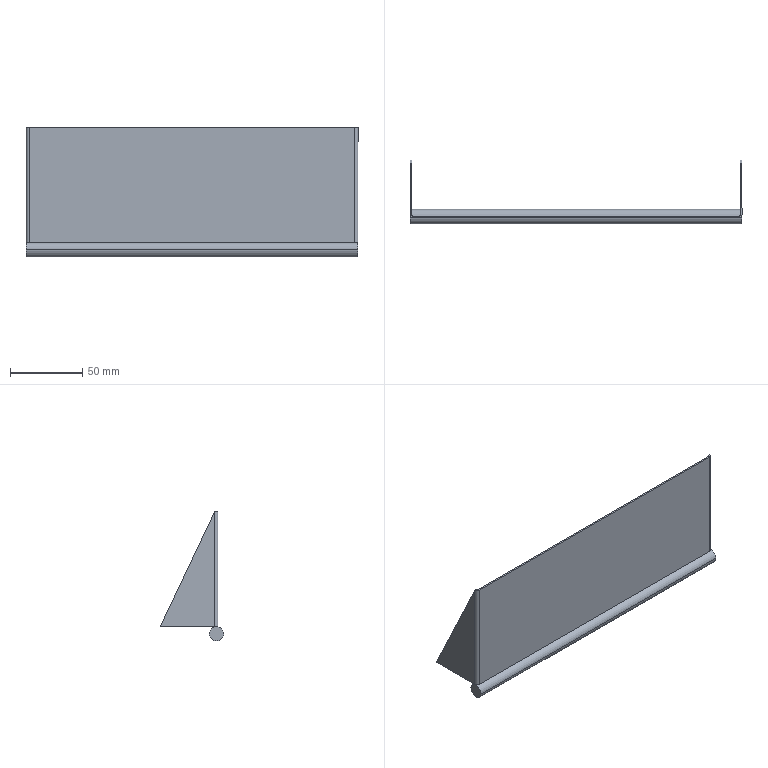Part | SolidWorks | features ICE 2, EdgeFlange 1, FlatPattern 1, SMBaseFlange 1, SheetMetal 1 | 2 solids | 24 faces | box 230 x 44 x 90 mm | volume 43833 mm3 | plane 18 | cylinder 6 | commonest cylinder face diameters 2 x2 4.4 x2 10 x2
STEP:
#1=CARTESIAN_POINT('',(112.8,-1.2,-40.));
#2=VERTEX_POINT('',#1);
#3=CARTESIAN_POINT('',(112.8,-1.2,40.));
#4=VERTEX_POINT('',#3);
#5=CARTESIAN_POINT('',(112.8,-1.2,-40.));
#6=DIRECTION('',(0.,0.,1.));
#7=VECTOR('',#6,1000.);
#8=LINE('',#5,#7);
#9=EDGE_CURVE('',#2,#4,#8,.T.);
#10=ORIENTED_EDGE('',*,*,#9,.T.);
#11=CARTESIAN_POINT('',(-112.8,-1.2,40.));
#12=VERTEX_POINT('',#11);
#13=CARTESIAN_POINT('',(-115.,-1.2,40.));
#14=DIRECTION('',(1.,0.,0.));
#15=VECTOR('',#14,1000.);
#16=LINE('',#13,#15);
#17=EDGE_CURVE('',#12,#4,#16,.T.);
#18=ORIENTED_EDGE('',*,*,#17,.F.);
#19=CARTESIAN_POINT('',(-112.8,-1.2,-40.));
#20=VERTEX_POINT('',#19);
#21=CARTESIAN_POINT('',(-112.8,-1.2,40.));
#22=DIRECTION('',(0.,0.,-1.));
#23=VECTOR('',#22,1000.);
#24=LINE('',#21,#23);
#25=EDGE_CURVE('',#12,#20,#24,.T.);
#26=ORIENTED_EDGE('',*,*,#25,.T.);
#27=CARTESIAN_POINT('',(-115.,-1.2,-40.));
#28=DIRECTION('',(-1.,0.,0.));
#29=VECTOR('',#28,1000.);
#30=LINE('',#27,#29);
#31=EDGE_CURVE('',#2,#20,#30,.T.);
#32=ORIENTED_EDGE('',*,*,#31,.F.);
#33=EDGE_LOOP('',(#10,#18,#26,#32));
#34=FACE_OUTER_BOUND('',#33,.T.);
#35=CARTESIAN_POINT('',(0.,-1.2,0.));
#36=DIRECTION('',(0.,1.,0.));
#37=DIRECTION('',(0.,0.,1.));
#38=AXIS2_PLACEMENT_3D('',#35,#36,#37);
#39=PLANE('',#38);
#40=ADVANCED_FACE('',(#34),#39,.F.);
#41=CARTESIAN_POINT('',(-112.8,0.,40.));
#42=VERTEX_POINT('',#41);
#43=CARTESIAN_POINT('',(112.8,0.,40.));
#44=VERTEX_POINT('',#43);
#45=CARTESIAN_POINT('',(-115.,0.,40.));
#46=DIRECTION('',(1.,0.,0.));
#47=VECTOR('',#46,1000.);
#48=LINE('',#45,#47);
#49=EDGE_CURVE('',#42,#44,#48,.T.);
#50=ORIENTED_EDGE('',*,*,#49,.T.);
#51=CARTESIAN_POINT('',(112.8,0.,-40.));
#52=VERTEX_POINT('',#51);
#53=CARTESIAN_POINT('',(112.8,0.,-40.));
#54=DIRECTION('',(0.,0.,1.));
#55=VECTOR('',#54,1000.);
#56=LINE('',#53,#55);
#57=EDGE_CURVE('',#52,#44,#56,.T.);
#58=ORIENTED_EDGE('',*,*,#57,.F.);
#59=CARTESIAN_POINT('',(-112.8,0.,-40.));
#60=VERTEX_POINT('',#59);
#61=CARTESIAN_POINT('',(-115.,0.,-40.));
#62=DIRECTION('',(-1.,0.,0.));
#63=VECTOR('',#62,1000.);
#64=LINE('',#61,#63);
#65=EDGE_CURVE('',#52,#60,#64,.T.);
#66=ORIENTED_EDGE('',*,*,#65,.T.);
#67=CARTESIAN_POINT('',(-112.8,0.,40.));
#68=DIRECTION('',(0.,0.,-1.));
#69=VECTOR('',#68,1000.);
#70=LINE('',#67,#69);
#71=EDGE_CURVE('',#42,#60,#70,.T.);
#72=ORIENTED_EDGE('',*,*,#71,.F.);
#73=EDGE_LOOP('',(#50,#58,#66,#72));
#74=FACE_OUTER_BOUND('',#73,.T.);
#75=CARTESIAN_POINT('',(0.,0.,0.));
#76=DIRECTION('',(0.,1.,0.));
#77=DIRECTION('',(0.,0.,1.));
#78=AXIS2_PLACEMENT_3D('',#75,#76,#77);
#79=PLANE('',#78);
#80=ADVANCED_FACE('',(#74),#79,.T.);
#81=ORIENTED_EDGE('',*,*,#65,.F.);
#82=CARTESIAN_POINT('',(112.8,0.,-40.));
#83=DIRECTION('',(0.,-1.,0.));
#84=VECTOR('',#83,1000.);
#85=LINE('',#82,#84);
#86=EDGE_CURVE('',#52,#2,#85,.T.);
#87=ORIENTED_EDGE('',*,*,#86,.T.);
#88=ORIENTED_EDGE('',*,*,#31,.T.);
#89=CARTESIAN_POINT('',(-112.8,0.,-40.));
#90=DIRECTION('',(0.,-1.,0.));
#91=VECTOR('',#90,1000.);
#92=LINE('',#89,#91);
#93=EDGE_CURVE('',#60,#20,#92,.T.);
#94=ORIENTED_EDGE('',*,*,#93,.F.);
#95=EDGE_LOOP('',(#81,#87,#88,#94));
#96=FACE_OUTER_BOUND('',#95,.T.);
#97=CARTESIAN_POINT('',(-115.,-1.2,-40.));
#98=DIRECTION('',(0.,0.,-1.));
#99=DIRECTION('',(-1.,0.,0.));
#100=AXIS2_PLACEMENT_3D('',#97,#98,#99);
#101=PLANE('',#100);
#102=ADVANCED_FACE('',(#96),#101,.T.);
#103=CARTESIAN_POINT('',(112.8,0.,40.));
#104=DIRECTION('',(0.,-1.,0.));
#105=VECTOR('',#104,1000.);
#106=LINE('',#103,#105);
#107=EDGE_CURVE('',#44,#4,#106,.T.);
#108=ORIENTED_EDGE('',*,*,#107,.F.);
#109=ORIENTED_EDGE('',*,*,#49,.F.);
#110=CARTESIAN_POINT('',(-112.8,0.,40.));
#111=DIRECTION('',(0.,-1.,0.));
#112=VECTOR('',#111,1000.);
#113=LINE('',#110,#112);
#114=EDGE_CURVE('',#42,#12,#113,.T.);
#115=ORIENTED_EDGE('',*,*,#114,.T.);
#116=ORIENTED_EDGE('',*,*,#17,.T.);
#117=EDGE_LOOP('',(#108,#109,#115,#116));
#118=FACE_OUTER_BOUND('',#117,.T.);
#119=CARTESIAN_POINT('',(-115.,-1.2,40.));
#120=DIRECTION('',(0.,0.,1.));
#121=DIRECTION('',(1.,0.,0.));
#122=AXIS2_PLACEMENT_3D('',#119,#120,#121);
#123=PLANE('',#122);
#124=ADVANCED_FACE('',(#118),#123,.T.);
#125=CARTESIAN_POINT('',(-113.8,1.,-40.));
#126=VERTEX_POINT('',#125);
#127=CARTESIAN_POINT('',(-115.,1.,-40.));
#128=VERTEX_POINT('',#127);
#129=CARTESIAN_POINT('',(-115.,1.,-40.));
#130=DIRECTION('',(-1.,0.,0.));
#131=VECTOR('',#130,1000.);
#132=LINE('',#129,#131);
#133=EDGE_CURVE('',#126,#128,#132,.T.);
#134=ORIENTED_EDGE('',*,*,#133,.F.);
#135=CARTESIAN_POINT('',(-112.8,1.,-40.));
#136=DIRECTION('',(0.,0.,-1.));
#137=DIRECTION('',(1.,0.,0.));
#138=AXIS2_PLACEMENT_3D('',#135,#136,#137);
#139=CIRCLE('',#138,1.);
#140=EDGE_CURVE('',#60,#126,#139,.T.);
#141=ORIENTED_EDGE('',*,*,#140,.F.);
#142=ORIENTED_EDGE('',*,*,#93,.T.);
#143=CARTESIAN_POINT('',(-112.8,1.,-40.));
#144=DIRECTION('',(0.,0.,-1.));
#145=DIRECTION('',(1.,0.,0.));
#146=AXIS2_PLACEMENT_3D('',#143,#144,#145);
#147=CIRCLE('',#146,2.2);
#148=EDGE_CURVE('',#20,#128,#147,.T.);
#149=ORIENTED_EDGE('',*,*,#148,.T.);
#150=EDGE_LOOP('',(#134,#141,#142,#149));
#151=FACE_OUTER_BOUND('',#150,.T.);
#152=CARTESIAN_POINT('',(-112.8,1.,-40.));
#153=DIRECTION('',(0.,0.,-1.));
#154=DIRECTION('',(-1.,0.,0.));
#155=AXIS2_PLACEMENT_3D('',#152,#153,#154);
#156=PLANE('',#155);
#157=ADVANCED_FACE('',(#151),#156,.T.);
#158=CARTESIAN_POINT('',(-113.8,1.,40.));
#159=VERTEX_POINT('',#158);
#160=CARTESIAN_POINT('',(-112.8,1.,40.));
#161=DIRECTION('',(0.,0.,1.));
#162=DIRECTION('',(1.,0.,0.));
#163=AXIS2_PLACEMENT_3D('',#160,#161,#162);
#164=CIRCLE('',#163,1.);
#165=EDGE_CURVE('',#159,#42,#164,.T.);
#166=ORIENTED_EDGE('',*,*,#165,.F.);
#167=CARTESIAN_POINT('',(-115.,1.,40.));
#168=VERTEX_POINT('',#167);
#169=CARTESIAN_POINT('',(-113.8,1.,40.));
#170=DIRECTION('',(-1.,0.,0.));
#171=VECTOR('',#170,1000.);
#172=LINE('',#169,#171);
#173=EDGE_CURVE('',#159,#168,#172,.T.);
#174=ORIENTED_EDGE('',*,*,#173,.T.);
#175=CARTESIAN_POINT('',(-112.8,1.,40.));
#176=DIRECTION('',(0.,0.,1.));
#177=DIRECTION('',(1.,0.,0.));
#178=AXIS2_PLACEMENT_3D('',#175,#176,#177);
#179=CIRCLE('',#178,2.2);
#180=EDGE_CURVE('',#168,#12,#179,.T.);
#181=ORIENTED_EDGE('',*,*,#180,.T.);
#182=ORIENTED_EDGE('',*,*,#114,.F.);
#183=EDGE_LOOP('',(#166,#174,#181,#182));
#184=FACE_OUTER_BOUND('',#183,.T.);
#185=CARTESIAN_POINT('',(-112.8,1.,40.));
#186=DIRECTION('',(0.,0.,-1.));
#187=DIRECTION('',(-1.,0.,0.));
#188=AXIS2_PLACEMENT_3D('',#185,#186,#187);
#189=PLANE('',#188);
#190=ADVANCED_FACE('',(#184),#189,.F.);
#191=ORIENTED_EDGE('',*,*,#25,.F.);
#192=ORIENTED_EDGE('',*,*,#180,.F.);
#193=CARTESIAN_POINT('',(-115.,1.,-40.));
#194=DIRECTION('',(0.,0.,-1.));
#195=VECTOR('',#194,1000.);
#196=LINE('',#193,#195);
#197=EDGE_CURVE('',#168,#128,#196,.T.);
#198=ORIENTED_EDGE('',*,*,#197,.T.);
#199=ORIENTED_EDGE('',*,*,#148,.F.);
#200=EDGE_LOOP('',(#191,#192,#198,#199));
#201=FACE_OUTER_BOUND('',#200,.T.);
#202=CARTESIAN_POINT('',(-112.8,1.,40.));
#203=DIRECTION('',(0.,0.,1.));
#204=DIRECTION('',(-1.,0.,0.));
#205=AXIS2_PLACEMENT_3D('',#202,#203,#204);
#206=CYLINDRICAL_SURFACE('',#205,2.2);
#207=ADVANCED_FACE('',(#201),#206,.T.);
#208=ORIENTED_EDGE('',*,*,#71,.T.);
#209=ORIENTED_EDGE('',*,*,#140,.T.);
#210=CARTESIAN_POINT('',(-113.8,1.,-40.));
#211=DIRECTION('',(0.,0.,1.));
#212=VECTOR('',#211,1000.);
#213=LINE('',#210,#212);
#214=EDGE_CURVE('',#126,#159,#213,.T.);
#215=ORIENTED_EDGE('',*,*,#214,.T.);
#216=ORIENTED_EDGE('',*,*,#165,.T.);
#217=EDGE_LOOP('',(#208,#209,#215,#216));
#218=FACE_OUTER_BOUND('',#217,.T.);
#219=CARTESIAN_POINT('',(-112.8,1.,40.));
#220=DIRECTION('',(0.,0.,1.));
#221=DIRECTION('',(-1.,0.,0.));
#222=AXIS2_PLACEMENT_3D('',#219,#220,#221);
#223=CYLINDRICAL_SURFACE('',#222,1.);
#224=ADVANCED_FACE('',(#218),#223,.F.);
#225=ORIENTED_EDGE('',*,*,#133,.T.);
#226=CARTESIAN_POINT('',(-115.,38.8,-40.));
#227=VERTEX_POINT('',#226);
#228=CARTESIAN_POINT('',(-115.,0.,-40.));
#229=DIRECTION('',(0.,-1.,0.));
#230=VECTOR('',#229,1000.);
#231=LINE('',#228,#230);
#232=EDGE_CURVE('',#227,#128,#231,.T.);
#233=ORIENTED_EDGE('',*,*,#232,.F.);
#234=CARTESIAN_POINT('',(-113.8,38.8,-40.));
#235=VERTEX_POINT('',#234);
#236=CARTESIAN_POINT('',(-115.,38.8,-40.));
#237=DIRECTION('',(1.,0.,0.));
#238=VECTOR('',#237,1000.);
#239=LINE('',#236,#238);
#240=EDGE_CURVE('',#227,#235,#239,.T.);
#241=ORIENTED_EDGE('',*,*,#240,.T.);
#242=CARTESIAN_POINT('',(-113.8,0.,-40.));
#243=DIRECTION('',(0.,-1.,0.));
#244=VECTOR('',#243,1000.);
#245=LINE('',#242,#244);
#246=EDGE_CURVE('',#235,#126,#245,.T.);
#247=ORIENTED_EDGE('',*,*,#246,.T.);
#248=EDGE_LOOP('',(#225,#233,#241,#247));
#249=FACE_OUTER_BOUND('',#248,.T.);
#250=CARTESIAN_POINT('',(-115.,0.,-40.));
#251=DIRECTION('',(0.,0.,1.));
#252=DIRECTION('',(1.,0.,0.));
#253=AXIS2_PLACEMENT_3D('',#250,#251,#252);
#254=PLANE('',#253);
#255=ADVANCED_FACE('',(#249),#254,.F.);
#256=ORIENTED_EDGE('',*,*,#197,.F.);
#257=CARTESIAN_POINT('',(-115.,16.268,7.687));
#258=DIRECTION('',(0.,0.4272,-0.9042));
#259=VECTOR('',#258,1000.);
#260=LINE('',#257,#259);
#261=EDGE_CURVE('',#168,#227,#260,.T.);
#262=ORIENTED_EDGE('',*,*,#261,.T.);
#263=ORIENTED_EDGE('',*,*,#232,.T.);
#264=EDGE_LOOP('',(#256,#262,#263));
#265=FACE_OUTER_BOUND('',#264,.T.);
#266=CARTESIAN_POINT('',(-115.,0.,0.));
#267=DIRECTION('',(1.,0.,0.));
#268=DIRECTION('',(0.,1.,0.));
#269=AXIS2_PLACEMENT_3D('',#266,#267,#268);
#270=PLANE('',#269);
#271=ADVANCED_FACE('',(#265),#270,.F.);
#272=CARTESIAN_POINT('',(-113.8,16.268,7.687));
#273=DIRECTION('',(0.,0.4272,-0.9042));
#274=VECTOR('',#273,1000.);
#275=LINE('',#272,#274);
#276=EDGE_CURVE('',#159,#235,#275,.T.);
#277=ORIENTED_EDGE('',*,*,#276,.F.);
#278=ORIENTED_EDGE('',*,*,#214,.F.);
#279=ORIENTED_EDGE('',*,*,#246,.F.);
#280=EDGE_LOOP('',(#277,#278,#279));
#281=FACE_OUTER_BOUND('',#280,.T.);
#282=CARTESIAN_POINT('',(-113.8,0.,0.));
#283=DIRECTION('',(1.,0.,0.));
#284=DIRECTION('',(0.,1.,0.));
#285=AXIS2_PLACEMENT_3D('',#282,#283,#284);
#286=PLANE('',#285);
#287=ADVANCED_FACE('',(#281),#286,.T.);
#288=CARTESIAN_POINT('',(113.8,1.,40.));
#289=VERTEX_POINT('',#288);
#290=CARTESIAN_POINT('',(115.,1.,40.));
#291=VERTEX_POINT('',#290);
#292=CARTESIAN_POINT('',(115.,1.,40.));
#293=DIRECTION('',(1.,0.,0.));
#294=VECTOR('',#293,1000.);
#295=LINE('',#292,#294);
#296=EDGE_CURVE('',#289,#291,#295,.T.);
#297=ORIENTED_EDGE('',*,*,#296,.F.);
#298=CARTESIAN_POINT('',(112.8,1.,40.));
#299=DIRECTION('',(0.,0.,1.));
#300=DIRECTION('',(-1.,0.,0.));
#301=AXIS2_PLACEMENT_3D('',#298,#299,#300);
#302=CIRCLE('',#301,1.);
#303=EDGE_CURVE('',#44,#289,#302,.T.);
#304=ORIENTED_EDGE('',*,*,#303,.F.);
#305=ORIENTED_EDGE('',*,*,#107,.T.);
#306=CARTESIAN_POINT('',(112.8,1.,40.));
#307=DIRECTION('',(0.,0.,1.));
#308=DIRECTION('',(-1.,0.,0.));
#309=AXIS2_PLACEMENT_3D('',#306,#307,#308);
#310=CIRCLE('',#309,2.2);
#311=EDGE_CURVE('',#4,#291,#310,.T.);
#312=ORIENTED_EDGE('',*,*,#311,.T.);
#313=EDGE_LOOP('',(#297,#304,#305,#312));
#314=FACE_OUTER_BOUND('',#313,.T.);
#315=CARTESIAN_POINT('',(112.8,1.,40.));
#316=DIRECTION('',(0.,0.,1.));
#317=DIRECTION('',(1.,0.,0.));
#318=AXIS2_PLACEMENT_3D('',#315,#316,#317);
#319=PLANE('',#318);
#320=ADVANCED_FACE('',(#314),#319,.T.);
#321=CARTESIAN_POINT('',(113.8,1.,-40.));
#322=VERTEX_POINT('',#321);
#323=CARTESIAN_POINT('',(112.8,1.,-40.));
#324=DIRECTION('',(0.,0.,-1.));
#325=DIRECTION('',(-1.,0.,0.));
#326=AXIS2_PLACEMENT_3D('',#323,#324,#325);
#327=CIRCLE('',#326,1.);
#328=EDGE_CURVE('',#322,#52,#327,.T.);
#329=ORIENTED_EDGE('',*,*,#328,.F.);
#330=CARTESIAN_POINT('',(115.,1.,-40.));
#331=VERTEX_POINT('',#330);
#332=CARTESIAN_POINT('',(113.8,1.,-40.));
#333=DIRECTION('',(1.,0.,0.));
#334=VECTOR('',#333,1000.);
#335=LINE('',#332,#334);
#336=EDGE_CURVE('',#322,#331,#335,.T.);
#337=ORIENTED_EDGE('',*,*,#336,.T.);
#338=CARTESIAN_POINT('',(112.8,1.,-40.));
#339=DIRECTION('',(0.,0.,-1.));
#340=DIRECTION('',(-1.,0.,0.));
#341=AXIS2_PLACEMENT_3D('',#338,#339,#340);
#342=CIRCLE('',#341,2.2);
#343=EDGE_CURVE('',#331,#2,#342,.T.);
#344=ORIENTED_EDGE('',*,*,#343,.T.);
#345=ORIENTED_EDGE('',*,*,#86,.F.);
#346=EDGE_LOOP('',(#329,#337,#344,#345));
#347=FACE_OUTER_BOUND('',#346,.T.);
#348=CARTESIAN_POINT('',(112.8,1.,-40.));
#349=DIRECTION('',(0.,0.,1.));
#350=DIRECTION('',(1.,0.,0.));
#351=AXIS2_PLACEMENT_3D('',#348,#349,#350);
#352=PLANE('',#351);
#353=ADVANCED_FACE('',(#347),#352,.F.);
#354=ORIENTED_EDGE('',*,*,#9,.F.);
#355=ORIENTED_EDGE('',*,*,#343,.F.);
#356=CARTESIAN_POINT('',(115.,1.,40.));
#357=DIRECTION('',(0.,0.,1.));
#358=VECTOR('',#357,1000.);
#359=LINE('',#356,#358);
#360=EDGE_CURVE('',#331,#291,#359,.T.);
#361=ORIENTED_EDGE('',*,*,#360,.T.);
#362=ORIENTED_EDGE('',*,*,#311,.F.);
#363=EDGE_LOOP('',(#354,#355,#361,#362));
#364=FACE_OUTER_BOUND('',#363,.T.);
#365=CARTESIAN_POINT('',(112.8,1.,-40.));
#366=DIRECTION('',(0.,0.,-1.));
#367=DIRECTION('',(1.,0.,0.));
#368=AXIS2_PLACEMENT_3D('',#365,#366,#367);
#369=CYLINDRICAL_SURFACE('',#368,2.2);
#370=ADVANCED_FACE('',(#364),#369,.T.);
#371=ORIENTED_EDGE('',*,*,#57,.T.);
#372=ORIENTED_EDGE('',*,*,#303,.T.);
#373=CARTESIAN_POINT('',(113.8,1.,40.));
#374=DIRECTION('',(0.,0.,-1.));
#375=VECTOR('',#374,1000.);
#376=LINE('',#373,#375);
#377=EDGE_CURVE('',#289,#322,#376,.T.);
#378=ORIENTED_EDGE('',*,*,#377,.T.);
#379=ORIENTED_EDGE('',*,*,#328,.T.);
#380=EDGE_LOOP('',(#371,#372,#378,#379));
#381=FACE_OUTER_BOUND('',#380,.T.);
#382=CARTESIAN_POINT('',(112.8,1.,-40.));
#383=DIRECTION('',(0.,0.,-1.));
#384=DIRECTION('',(1.,0.,0.));
#385=AXIS2_PLACEMENT_3D('',#382,#383,#384);
#386=CYLINDRICAL_SURFACE('',#385,1.);
#387=ADVANCED_FACE('',(#381),#386,.F.);
#388=ORIENTED_EDGE('',*,*,#336,.F.);
#389=CARTESIAN_POINT('',(113.8,38.8,-40.));
#390=VERTEX_POINT('',#389);
#391=CARTESIAN_POINT('',(113.8,38.8,-40.));
#392=DIRECTION('',(0.,1.,0.));
#393=VECTOR('',#392,1000.);
#394=LINE('',#391,#393);
#395=EDGE_CURVE('',#322,#390,#394,.T.);
#396=ORIENTED_EDGE('',*,*,#395,.T.);
#397=CARTESIAN_POINT('',(115.,38.8,-40.));
#398=VERTEX_POINT('',#397);
#399=CARTESIAN_POINT('',(115.,38.8,-40.));
#400=DIRECTION('',(-1.,0.,0.));
#401=VECTOR('',#400,1000.);
#402=LINE('',#399,#401);
#403=EDGE_CURVE('',#398,#390,#402,.T.);
#404=ORIENTED_EDGE('',*,*,#403,.F.);
#405=CARTESIAN_POINT('',(115.,0.,-40.));
#406=DIRECTION('',(0.,1.,0.));
#407=VECTOR('',#406,1000.);
#408=LINE('',#405,#407);
#409=EDGE_CURVE('',#331,#398,#408,.T.);
#410=ORIENTED_EDGE('',*,*,#409,.F.);
#411=EDGE_LOOP('',(#388,#396,#404,#410));
#412=FACE_OUTER_BOUND('',#411,.T.);
#413=CARTESIAN_POINT('',(115.,38.8,-40.));
#414=DIRECTION('',(0.,0.,1.));
#415=DIRECTION('',(0.,-1.,0.));
#416=AXIS2_PLACEMENT_3D('',#413,#414,#415);
#417=PLANE('',#416);
#418=ADVANCED_FACE('',(#412),#417,.F.);
#419=ORIENTED_EDGE('',*,*,#409,.T.);
#420=CARTESIAN_POINT('',(115.,1.,40.));
#421=DIRECTION('',(0.,-0.4272,0.9042));
#422=VECTOR('',#421,1000.);
#423=LINE('',#420,#422);
#424=EDGE_CURVE('',#398,#291,#423,.T.);
#425=ORIENTED_EDGE('',*,*,#424,.T.);
#426=ORIENTED_EDGE('',*,*,#360,.F.);
#427=EDGE_LOOP('',(#419,#425,#426));
#428=FACE_OUTER_BOUND('',#427,.T.);
#429=CARTESIAN_POINT('',(115.,0.,0.));
#430=DIRECTION('',(-1.,0.,0.));
#431=DIRECTION('',(0.,-1.,0.));
#432=AXIS2_PLACEMENT_3D('',#429,#430,#431);
#433=PLANE('',#432);
#434=ADVANCED_FACE('',(#428),#433,.F.);
#435=CARTESIAN_POINT('',(113.8,16.268,7.687));
#436=DIRECTION('',(0.,-0.4272,0.9042));
#437=VECTOR('',#436,1000.);
#438=LINE('',#435,#437);
#439=EDGE_CURVE('',#390,#289,#438,.T.);
#440=ORIENTED_EDGE('',*,*,#439,.F.);
#441=ORIENTED_EDGE('',*,*,#395,.F.);
#442=ORIENTED_EDGE('',*,*,#377,.F.);
#443=EDGE_LOOP('',(#440,#441,#442));
#444=FACE_OUTER_BOUND('',#443,.T.);
#445=CARTESIAN_POINT('',(113.8,0.,0.));
#446=DIRECTION('',(-1.,0.,0.));
#447=DIRECTION('',(0.,-1.,0.));
#448=AXIS2_PLACEMENT_3D('',#445,#446,#447);
#449=PLANE('',#448);
#450=ADVANCED_FACE('',(#444),#449,.T.);
#451=ORIENTED_EDGE('',*,*,#439,.T.);
#452=ORIENTED_EDGE('',*,*,#296,.T.);
#453=ORIENTED_EDGE('',*,*,#424,.F.);
#454=ORIENTED_EDGE('',*,*,#403,.T.);
#455=EDGE_LOOP('',(#451,#452,#453,#454));
#456=FACE_OUTER_BOUND('',#455,.T.);
#457=CARTESIAN_POINT('',(115.,1.,40.));
#458=DIRECTION('',(0.,-0.9042,-0.4272));
#459=DIRECTION('',(0.,0.4272,-0.9042));
#460=AXIS2_PLACEMENT_3D('',#457,#458,#459);
#461=PLANE('',#460);
#462=ADVANCED_FACE('',(#456),#461,.F.);
#463=ORIENTED_EDGE('',*,*,#173,.F.);
#464=ORIENTED_EDGE('',*,*,#276,.T.);
#465=ORIENTED_EDGE('',*,*,#240,.F.);
#466=ORIENTED_EDGE('',*,*,#261,.F.);
#467=EDGE_LOOP('',(#463,#464,#465,#466));
#468=FACE_OUTER_BOUND('',#467,.T.);
#469=CARTESIAN_POINT('',(115.,1.,40.));
#470=DIRECTION('',(0.,-0.9042,-0.4272));
#471=DIRECTION('',(0.,0.4272,-0.9042));
#472=AXIS2_PLACEMENT_3D('',#469,#470,#471);
#473=PLANE('',#472);
#474=ADVANCED_FACE('',(#468),#473,.F.);
#475=CLOSED_SHELL('',(#40,#80,#102,#124,#157,#190,#207,#224,#255,#271,#287,#320,#353,#370,#387,#418,#434,#450,#462,#474));
#476=MANIFOLD_SOLID_BREP('',#475);
#477=CARTESIAN_POINT('',(115.,-5.2,-45.));
#478=VERTEX_POINT('',#477);
#479=CARTESIAN_POINT('',(115.,4.8,-45.));
#480=VERTEX_POINT('',#479);
#481=CARTESIAN_POINT('',(115.,-0.2,-45.));
#482=DIRECTION('',(-1.,0.,0.));
#483=DIRECTION('',(0.,-1.,0.));
#484=AXIS2_PLACEMENT_3D('',#481,#482,#483);
#485=CIRCLE('',#484,5.);
#486=EDGE_CURVE('',#478,#480,#485,.T.);
#487=ORIENTED_EDGE('',*,*,#486,.T.);
#488=CARTESIAN_POINT('',(-115.,4.8,-45.));
#489=VERTEX_POINT('',#488);
#490=CARTESIAN_POINT('',(115.,4.8,-45.));
#491=DIRECTION('',(-1.,0.,0.));
#492=VECTOR('',#491,1000.);
#493=LINE('',#490,#492);
#494=EDGE_CURVE('',#480,#489,#493,.T.);
#495=ORIENTED_EDGE('',*,*,#494,.T.);
#496=CARTESIAN_POINT('',(-115.,-5.2,-45.));
#497=VERTEX_POINT('',#496);
#498=CARTESIAN_POINT('',(-115.,-0.2,-45.));
#499=DIRECTION('',(-1.,0.,0.));
#500=DIRECTION('',(0.,-1.,0.));
#501=AXIS2_PLACEMENT_3D('',#498,#499,#500);
#502=CIRCLE('',#501,5.);
#503=EDGE_CURVE('',#497,#489,#502,.T.);
#504=ORIENTED_EDGE('',*,*,#503,.F.);
#505=CARTESIAN_POINT('',(115.,-5.2,-45.));
#506=DIRECTION('',(-1.,0.,0.));
#507=VECTOR('',#506,1000.);
#508=LINE('',#505,#507);
#509=EDGE_CURVE('',#478,#497,#508,.T.);
#510=ORIENTED_EDGE('',*,*,#509,.F.);
#511=EDGE_LOOP('',(#487,#495,#504,#510));
#512=FACE_OUTER_BOUND('',#511,.T.);
#513=CARTESIAN_POINT('',(115.,-0.2,-45.));
#514=DIRECTION('',(-1.,0.,0.));
#515=DIRECTION('',(0.,-1.,0.));
#516=AXIS2_PLACEMENT_3D('',#513,#514,#515);
#517=CYLINDRICAL_SURFACE('',#516,5.);
#518=ADVANCED_FACE('',(#512),#517,.T.);
#519=ORIENTED_EDGE('',*,*,#494,.F.);
#520=CARTESIAN_POINT('',(115.,-0.2,-45.));
#521=DIRECTION('',(-1.,0.,0.));
#522=DIRECTION('',(0.,-1.,0.));
#523=AXIS2_PLACEMENT_3D('',#520,#521,#522);
#524=CIRCLE('',#523,5.);
#525=EDGE_CURVE('',#480,#478,#524,.T.);
#526=ORIENTED_EDGE('',*,*,#525,.T.);
#527=ORIENTED_EDGE('',*,*,#509,.T.);
#528=CARTESIAN_POINT('',(-115.,-0.2,-45.));
#529=DIRECTION('',(-1.,0.,0.));
#530=DIRECTION('',(0.,-1.,0.));
#531=AXIS2_PLACEMENT_3D('',#528,#529,#530);
#532=CIRCLE('',#531,5.);
#533=EDGE_CURVE('',#489,#497,#532,.T.);
#534=ORIENTED_EDGE('',*,*,#533,.F.);
#535=EDGE_LOOP('',(#519,#526,#527,#534));
#536=FACE_OUTER_BOUND('',#535,.T.);
#537=CARTESIAN_POINT('',(115.,-0.2,-45.));
#538=DIRECTION('',(-1.,0.,0.));
#539=DIRECTION('',(0.,-1.,0.));
#540=AXIS2_PLACEMENT_3D('',#537,#538,#539);
#541=CYLINDRICAL_SURFACE('',#540,5.);
#542=ADVANCED_FACE('',(#536),#541,.T.);
#543=ORIENTED_EDGE('',*,*,#486,.F.);
#544=ORIENTED_EDGE('',*,*,#525,.F.);
#545=EDGE_LOOP('',(#543,#544));
#546=FACE_OUTER_BOUND('',#545,.T.);
#547=CARTESIAN_POINT('',(115.,-0.2,-45.));
#548=DIRECTION('',(-1.,0.,0.));
#549=DIRECTION('',(0.,-1.,0.));
#550=AXIS2_PLACEMENT_3D('',#547,#548,#549);
#551=PLANE('',#550);
#552=ADVANCED_FACE('',(#546),#551,.F.);
#553=ORIENTED_EDGE('',*,*,#503,.T.);
#554=ORIENTED_EDGE('',*,*,#533,.T.);
#555=EDGE_LOOP('',(#553,#554));
#556=FACE_OUTER_BOUND('',#555,.T.);
#557=CARTESIAN_POINT('',(-115.,-0.2,-45.));
#558=DIRECTION('',(-1.,0.,0.));
#559=DIRECTION('',(0.,-1.,0.));
#560=AXIS2_PLACEMENT_3D('',#557,#558,#559);
#561=PLANE('',#560);
#562=ADVANCED_FACE('',(#556),#561,.T.);
#563=CLOSED_SHELL('',(#518,#542,#552,#562));
#564=MANIFOLD_SOLID_BREP('',#563);
#565=CARTESIAN_POINT('',(0.,0.,0.));
#566=DIRECTION('',(0.,0.,1.));
#567=DIRECTION('',(1.,0.,0.));
#568=AXIS2_PLACEMENT_3D('',#565,#566,#567);
#569=(LENGTH_UNIT()NAMED_UNIT(*)SI_UNIT(.MILLI.,.METRE.));
#570=UNCERTAINTY_MEASURE_WITH_UNIT(LENGTH_MEASURE(0.00001),#569,'','');
#571=(NAMED_UNIT(*)PLANE_ANGLE_UNIT()SI_UNIT($,.RADIAN.));
#572=(NAMED_UNIT(*)SI_UNIT($,.STERADIAN.)SOLID_ANGLE_UNIT());
#573=(GEOMETRIC_REPRESENTATION_CONTEXT(3)GLOBAL_UNCERTAINTY_ASSIGNED_CONTEXT((#570))GLOBAL_UNIT_ASSIGNED_CONTEXT((#569,#571,#572))REPRESENTATION_CONTEXT('',''));
#574=ADVANCED_BREP_SHAPE_REPRESENTATION('',(#476,#564,#568),#573);